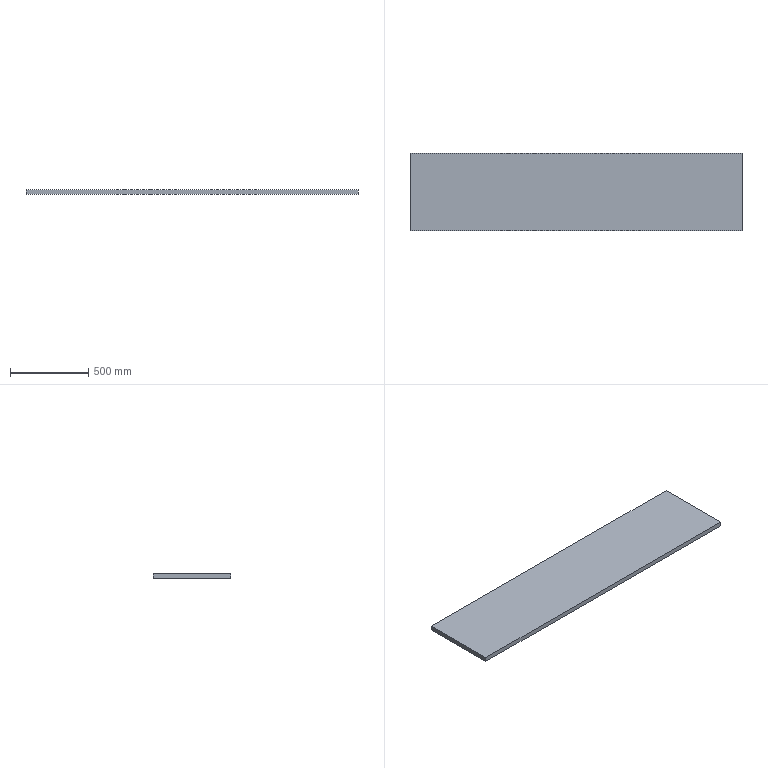Part | SolidWorks | features Extrusion 1 | 1 solid | 6 faces | box 2118 x 492 x 30 mm | volume 31261680 mm3 | plane 6
STEP:
#1=CARTESIAN_POINT('',(0.,492.,0.));
#2=VERTEX_POINT('',#1);
#3=CARTESIAN_POINT('',(0.,0.,0.));
#4=VERTEX_POINT('',#3);
#5=CARTESIAN_POINT('',(0.,0.,0.));
#6=DIRECTION('',(0.,-1.,0.));
#7=VECTOR('',#6,1000.);
#8=LINE('',#5,#7);
#9=EDGE_CURVE('',#2,#4,#8,.T.);
#10=ORIENTED_EDGE('',*,*,#9,.T.);
#11=CARTESIAN_POINT('',(0.,0.,30.));
#12=VERTEX_POINT('',#11);
#13=CARTESIAN_POINT('',(0.,0.,30.));
#14=DIRECTION('',(0.,0.,-1.));
#15=VECTOR('',#14,1000.);
#16=LINE('',#13,#15);
#17=EDGE_CURVE('',#12,#4,#16,.T.);
#18=ORIENTED_EDGE('',*,*,#17,.F.);
#19=CARTESIAN_POINT('',(0.,492.,30.));
#20=VERTEX_POINT('',#19);
#21=CARTESIAN_POINT('',(0.,0.,30.));
#22=DIRECTION('',(0.,-1.,0.));
#23=VECTOR('',#22,1000.);
#24=LINE('',#21,#23);
#25=EDGE_CURVE('',#20,#12,#24,.T.);
#26=ORIENTED_EDGE('',*,*,#25,.F.);
#27=CARTESIAN_POINT('',(0.,492.,30.));
#28=DIRECTION('',(0.,0.,-1.));
#29=VECTOR('',#28,1000.);
#30=LINE('',#27,#29);
#31=EDGE_CURVE('',#20,#2,#30,.T.);
#32=ORIENTED_EDGE('',*,*,#31,.T.);
#33=EDGE_LOOP('',(#10,#18,#26,#32));
#34=FACE_OUTER_BOUND('',#33,.T.);
#35=CARTESIAN_POINT('',(0.,0.,30.));
#36=DIRECTION('',(1.,0.,0.));
#37=DIRECTION('',(0.,0.,-1.));
#38=AXIS2_PLACEMENT_3D('',#35,#36,#37);
#39=PLANE('',#38);
#40=ADVANCED_FACE('',(#34),#39,.F.);
#41=CARTESIAN_POINT('',(2118.,0.,0.));
#42=VERTEX_POINT('',#41);
#43=CARTESIAN_POINT('',(0.,0.,0.));
#44=DIRECTION('',(1.,0.,0.));
#45=VECTOR('',#44,1000.);
#46=LINE('',#43,#45);
#47=EDGE_CURVE('',#4,#42,#46,.T.);
#48=ORIENTED_EDGE('',*,*,#47,.T.);
#49=CARTESIAN_POINT('',(2118.,0.,30.));
#50=VERTEX_POINT('',#49);
#51=CARTESIAN_POINT('',(2118.,0.,30.));
#52=DIRECTION('',(0.,0.,-1.));
#53=VECTOR('',#52,1000.);
#54=LINE('',#51,#53);
#55=EDGE_CURVE('',#50,#42,#54,.T.);
#56=ORIENTED_EDGE('',*,*,#55,.F.);
#57=CARTESIAN_POINT('',(0.,0.,30.));
#58=DIRECTION('',(1.,0.,0.));
#59=VECTOR('',#58,1000.);
#60=LINE('',#57,#59);
#61=EDGE_CURVE('',#12,#50,#60,.T.);
#62=ORIENTED_EDGE('',*,*,#61,.F.);
#63=ORIENTED_EDGE('',*,*,#17,.T.);
#64=EDGE_LOOP('',(#48,#56,#62,#63));
#65=FACE_OUTER_BOUND('',#64,.T.);
#66=CARTESIAN_POINT('',(0.,0.,30.));
#67=DIRECTION('',(0.,1.,0.));
#68=DIRECTION('',(0.,0.,1.));
#69=AXIS2_PLACEMENT_3D('',#66,#67,#68);
#70=PLANE('',#69);
#71=ADVANCED_FACE('',(#65),#70,.F.);
#72=CARTESIAN_POINT('',(2118.,492.,0.));
#73=VERTEX_POINT('',#72);
#74=CARTESIAN_POINT('',(2118.,0.,0.));
#75=DIRECTION('',(0.,1.,0.));
#76=VECTOR('',#75,1000.);
#77=LINE('',#74,#76);
#78=EDGE_CURVE('',#42,#73,#77,.T.);
#79=ORIENTED_EDGE('',*,*,#78,.T.);
#80=CARTESIAN_POINT('',(2118.,492.,30.));
#81=VERTEX_POINT('',#80);
#82=CARTESIAN_POINT('',(2118.,492.,30.));
#83=DIRECTION('',(0.,0.,-1.));
#84=VECTOR('',#83,1000.);
#85=LINE('',#82,#84);
#86=EDGE_CURVE('',#81,#73,#85,.T.);
#87=ORIENTED_EDGE('',*,*,#86,.F.);
#88=CARTESIAN_POINT('',(2118.,0.,30.));
#89=DIRECTION('',(0.,1.,0.));
#90=VECTOR('',#89,1000.);
#91=LINE('',#88,#90);
#92=EDGE_CURVE('',#50,#81,#91,.T.);
#93=ORIENTED_EDGE('',*,*,#92,.F.);
#94=ORIENTED_EDGE('',*,*,#55,.T.);
#95=EDGE_LOOP('',(#79,#87,#93,#94));
#96=FACE_OUTER_BOUND('',#95,.T.);
#97=CARTESIAN_POINT('',(2118.,0.,30.));
#98=DIRECTION('',(-1.,0.,0.));
#99=DIRECTION('',(0.,0.,1.));
#100=AXIS2_PLACEMENT_3D('',#97,#98,#99);
#101=PLANE('',#100);
#102=ADVANCED_FACE('',(#96),#101,.F.);
#103=CARTESIAN_POINT('',(0.,492.,0.));
#104=DIRECTION('',(-1.,0.,0.));
#105=VECTOR('',#104,1000.);
#106=LINE('',#103,#105);
#107=EDGE_CURVE('',#73,#2,#106,.T.);
#108=ORIENTED_EDGE('',*,*,#107,.T.);
#109=ORIENTED_EDGE('',*,*,#31,.F.);
#110=CARTESIAN_POINT('',(0.,492.,30.));
#111=DIRECTION('',(-1.,0.,0.));
#112=VECTOR('',#111,1000.);
#113=LINE('',#110,#112);
#114=EDGE_CURVE('',#81,#20,#113,.T.);
#115=ORIENTED_EDGE('',*,*,#114,.F.);
#116=ORIENTED_EDGE('',*,*,#86,.T.);
#117=EDGE_LOOP('',(#108,#109,#115,#116));
#118=FACE_OUTER_BOUND('',#117,.T.);
#119=CARTESIAN_POINT('',(0.,492.,30.));
#120=DIRECTION('',(0.,-1.,0.));
#121=DIRECTION('',(0.,0.,-1.));
#122=AXIS2_PLACEMENT_3D('',#119,#120,#121);
#123=PLANE('',#122);
#124=ADVANCED_FACE('',(#118),#123,.F.);
#125=ORIENTED_EDGE('',*,*,#25,.T.);
#126=ORIENTED_EDGE('',*,*,#61,.T.);
#127=ORIENTED_EDGE('',*,*,#92,.T.);
#128=ORIENTED_EDGE('',*,*,#114,.T.);
#129=EDGE_LOOP('',(#125,#126,#127,#128));
#130=FACE_OUTER_BOUND('',#129,.T.);
#131=CARTESIAN_POINT('',(0.,0.,30.));
#132=DIRECTION('',(0.,0.,-1.));
#133=DIRECTION('',(-1.,0.,0.));
#134=AXIS2_PLACEMENT_3D('',#131,#132,#133);
#135=PLANE('',#134);
#136=ADVANCED_FACE('',(#130),#135,.F.);
#137=ORIENTED_EDGE('',*,*,#9,.F.);
#138=ORIENTED_EDGE('',*,*,#107,.F.);
#139=ORIENTED_EDGE('',*,*,#78,.F.);
#140=ORIENTED_EDGE('',*,*,#47,.F.);
#141=EDGE_LOOP('',(#137,#138,#139,#140));
#142=FACE_OUTER_BOUND('',#141,.T.);
#143=CARTESIAN_POINT('',(0.,0.,0.));
#144=DIRECTION('',(0.,0.,-1.));
#145=DIRECTION('',(-1.,0.,0.));
#146=AXIS2_PLACEMENT_3D('',#143,#144,#145);
#147=PLANE('',#146);
#148=ADVANCED_FACE('',(#142),#147,.T.);
#149=CLOSED_SHELL('',(#40,#71,#102,#124,#136,#148));
#150=MANIFOLD_SOLID_BREP('',#149);
#151=CARTESIAN_POINT('',(0.,0.,0.));
#152=DIRECTION('',(0.,0.,1.));
#153=DIRECTION('',(1.,0.,0.));
#154=AXIS2_PLACEMENT_3D('',#151,#152,#153);
#155=(LENGTH_UNIT()NAMED_UNIT(*)SI_UNIT(.MILLI.,.METRE.));
#156=UNCERTAINTY_MEASURE_WITH_UNIT(LENGTH_MEASURE(0.00001),#155,'','');
#157=(NAMED_UNIT(*)PLANE_ANGLE_UNIT()SI_UNIT($,.RADIAN.));
#158=(NAMED_UNIT(*)SI_UNIT($,.STERADIAN.)SOLID_ANGLE_UNIT());
#159=(GEOMETRIC_REPRESENTATION_CONTEXT(3)GLOBAL_UNCERTAINTY_ASSIGNED_CONTEXT((#156))GLOBAL_UNIT_ASSIGNED_CONTEXT((#155,#157,#158))REPRESENTATION_CONTEXT('',''));
#160=ADVANCED_BREP_SHAPE_REPRESENTATION('',(#150,#154),#159);